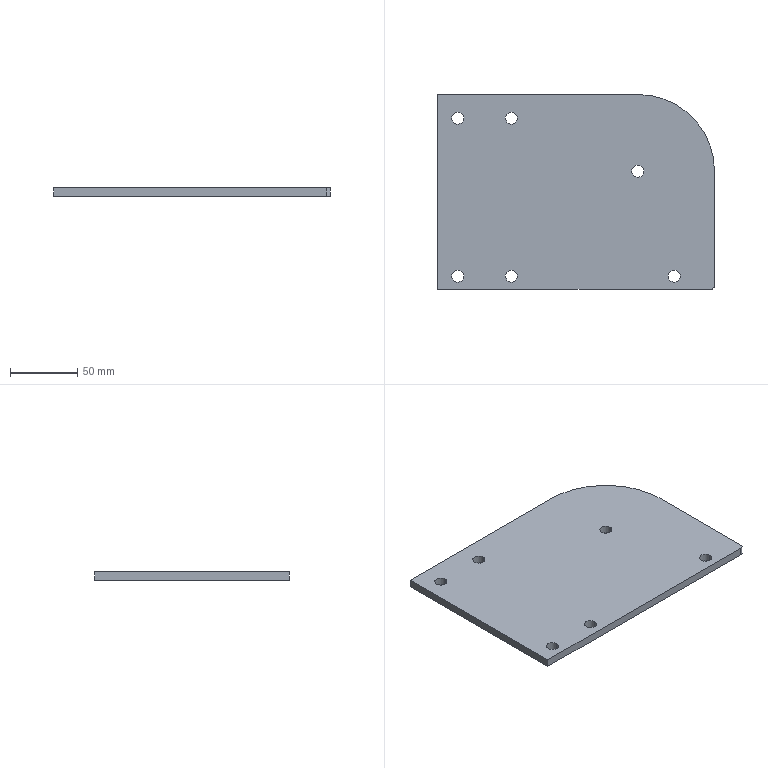Part | SolidWorks | features ICE 7, Fillet 6, Chamfer 1, Extrusion 1, HoleWzd 1 | 1 solid | 20 faces | box 206 x 145 x 6 mm | volume 172735 mm3 | cylinder 14 | plane 6 | commonest cylinder face diameters 9 x12 6 x1 114 x1
STEP:
#1=CARTESIAN_POINT('',(68.5,-62.5,6.));
#2=VERTEX_POINT('',#1);
#3=CARTESIAN_POINT('',(77.5,-62.5,6.));
#4=VERTEX_POINT('',#3);
#5=CARTESIAN_POINT('',(73.,-62.5,6.));
#6=DIRECTION('',(0.,0.,1.));
#7=DIRECTION('',(1.,0.,0.));
#8=AXIS2_PLACEMENT_3D('',#5,#6,#7);
#9=CIRCLE('',#8,4.5);
#10=EDGE_CURVE('',#2,#4,#9,.T.);
#11=ORIENTED_EDGE('',*,*,#10,.T.);
#12=CARTESIAN_POINT('',(77.5,-62.5,0.));
#13=VERTEX_POINT('',#12);
#14=CARTESIAN_POINT('',(77.5,-62.5,10.));
#15=DIRECTION('',(0.,0.,-1.));
#16=VECTOR('',#15,1000.);
#17=LINE('',#14,#16);
#18=EDGE_CURVE('',#4,#13,#17,.T.);
#19=ORIENTED_EDGE('',*,*,#18,.T.);
#20=CARTESIAN_POINT('',(68.5,-62.5,0.));
#21=VERTEX_POINT('',#20);
#22=CARTESIAN_POINT('',(73.,-62.5,0.));
#23=DIRECTION('',(0.,0.,-1.));
#24=DIRECTION('',(-1.,0.,0.));
#25=AXIS2_PLACEMENT_3D('',#22,#23,#24);
#26=CIRCLE('',#25,4.5);
#27=EDGE_CURVE('',#13,#21,#26,.T.);
#28=ORIENTED_EDGE('',*,*,#27,.T.);
#29=CARTESIAN_POINT('',(68.5,-62.5,10.));
#30=DIRECTION('',(0.,0.,-1.));
#31=VECTOR('',#30,1000.);
#32=LINE('',#29,#31);
#33=EDGE_CURVE('',#2,#21,#32,.T.);
#34=ORIENTED_EDGE('',*,*,#33,.F.);
#35=EDGE_LOOP('',(#11,#19,#28,#34));
#36=FACE_OUTER_BOUND('',#35,.T.);
#37=CARTESIAN_POINT('',(73.,-62.5,10.));
#38=DIRECTION('',(0.,0.,-1.));
#39=DIRECTION('',(-1.,0.,0.));
#40=AXIS2_PLACEMENT_3D('',#37,#38,#39);
#41=CYLINDRICAL_SURFACE('',#40,4.5);
#42=ADVANCED_FACE('',(#36),#41,.F.);
#43=CARTESIAN_POINT('',(41.5,15.5,0.));
#44=VERTEX_POINT('',#43);
#45=CARTESIAN_POINT('',(50.5,15.5,0.));
#46=VERTEX_POINT('',#45);
#47=CARTESIAN_POINT('',(46.,15.5,0.));
#48=DIRECTION('',(0.,0.,1.));
#49=DIRECTION('',(1.,0.,0.));
#50=AXIS2_PLACEMENT_3D('',#47,#48,#49);
#51=CIRCLE('',#50,4.5);
#52=EDGE_CURVE('',#44,#46,#51,.T.);
#53=ORIENTED_EDGE('',*,*,#52,.F.);
#54=CARTESIAN_POINT('',(41.5,15.5,6.));
#55=VERTEX_POINT('',#54);
#56=CARTESIAN_POINT('',(41.5,15.5,0.));
#57=DIRECTION('',(0.,0.,1.));
#58=VECTOR('',#57,1000.);
#59=LINE('',#56,#58);
#60=EDGE_CURVE('',#44,#55,#59,.T.);
#61=ORIENTED_EDGE('',*,*,#60,.T.);
#62=CARTESIAN_POINT('',(50.5,15.5,6.));
#63=VERTEX_POINT('',#62);
#64=CARTESIAN_POINT('',(46.,15.5,6.));
#65=DIRECTION('',(0.,0.,1.));
#66=DIRECTION('',(1.,0.,0.));
#67=AXIS2_PLACEMENT_3D('',#64,#65,#66);
#68=CIRCLE('',#67,4.5);
#69=EDGE_CURVE('',#55,#63,#68,.T.);
#70=ORIENTED_EDGE('',*,*,#69,.T.);
#71=CARTESIAN_POINT('',(50.5,15.5,0.));
#72=DIRECTION('',(0.,0.,1.));
#73=VECTOR('',#72,1000.);
#74=LINE('',#71,#73);
#75=EDGE_CURVE('',#46,#63,#74,.T.);
#76=ORIENTED_EDGE('',*,*,#75,.F.);
#77=EDGE_LOOP('',(#53,#61,#70,#76));
#78=FACE_OUTER_BOUND('',#77,.T.);
#79=CARTESIAN_POINT('',(46.,15.5,0.));
#80=DIRECTION('',(0.,0.,1.));
#81=DIRECTION('',(1.,0.,0.));
#82=AXIS2_PLACEMENT_3D('',#79,#80,#81);
#83=CYLINDRICAL_SURFACE('',#82,4.5);
#84=ADVANCED_FACE('',(#78),#83,.F.);
#85=CARTESIAN_POINT('',(-52.5,-62.5,0.));
#86=VERTEX_POINT('',#85);
#87=CARTESIAN_POINT('',(-43.5,-62.5,0.));
#88=VERTEX_POINT('',#87);
#89=CARTESIAN_POINT('',(-48.,-62.5,0.));
#90=DIRECTION('',(0.,0.,1.));
#91=DIRECTION('',(1.,0.,0.));
#92=AXIS2_PLACEMENT_3D('',#89,#90,#91);
#93=CIRCLE('',#92,4.5);
#94=EDGE_CURVE('',#86,#88,#93,.T.);
#95=ORIENTED_EDGE('',*,*,#94,.F.);
#96=CARTESIAN_POINT('',(-52.5,-62.5,6.));
#97=VERTEX_POINT('',#96);
#98=CARTESIAN_POINT('',(-52.5,-62.5,0.));
#99=DIRECTION('',(0.,0.,1.));
#100=VECTOR('',#99,1000.);
#101=LINE('',#98,#100);
#102=EDGE_CURVE('',#86,#97,#101,.T.);
#103=ORIENTED_EDGE('',*,*,#102,.T.);
#104=CARTESIAN_POINT('',(-43.5,-62.5,6.));
#105=VERTEX_POINT('',#104);
#106=CARTESIAN_POINT('',(-48.,-62.5,6.));
#107=DIRECTION('',(0.,0.,1.));
#108=DIRECTION('',(1.,0.,0.));
#109=AXIS2_PLACEMENT_3D('',#106,#107,#108);
#110=CIRCLE('',#109,4.5);
#111=EDGE_CURVE('',#97,#105,#110,.T.);
#112=ORIENTED_EDGE('',*,*,#111,.T.);
#113=CARTESIAN_POINT('',(-43.5,-62.5,0.));
#114=DIRECTION('',(0.,0.,1.));
#115=VECTOR('',#114,1000.);
#116=LINE('',#113,#115);
#117=EDGE_CURVE('',#88,#105,#116,.T.);
#118=ORIENTED_EDGE('',*,*,#117,.F.);
#119=EDGE_LOOP('',(#95,#103,#112,#118));
#120=FACE_OUTER_BOUND('',#119,.T.);
#121=CARTESIAN_POINT('',(-48.,-62.5,0.));
#122=DIRECTION('',(0.,0.,1.));
#123=DIRECTION('',(1.,0.,0.));
#124=AXIS2_PLACEMENT_3D('',#121,#122,#123);
#125=CYLINDRICAL_SURFACE('',#124,4.5);
#126=ADVANCED_FACE('',(#120),#125,.F.);
#127=CARTESIAN_POINT('',(-92.5,-62.5,0.));
#128=VERTEX_POINT('',#127);
#129=CARTESIAN_POINT('',(-83.5,-62.5,0.));
#130=VERTEX_POINT('',#129);
#131=CARTESIAN_POINT('',(-88.,-62.5,0.));
#132=DIRECTION('',(0.,0.,1.));
#133=DIRECTION('',(1.,0.,0.));
#134=AXIS2_PLACEMENT_3D('',#131,#132,#133);
#135=CIRCLE('',#134,4.5);
#136=EDGE_CURVE('',#128,#130,#135,.T.);
#137=ORIENTED_EDGE('',*,*,#136,.F.);
#138=CARTESIAN_POINT('',(-92.5,-62.5,6.));
#139=VERTEX_POINT('',#138);
#140=CARTESIAN_POINT('',(-92.5,-62.5,0.));
#141=DIRECTION('',(0.,0.,1.));
#142=VECTOR('',#141,1000.);
#143=LINE('',#140,#142);
#144=EDGE_CURVE('',#128,#139,#143,.T.);
#145=ORIENTED_EDGE('',*,*,#144,.T.);
#146=CARTESIAN_POINT('',(-83.5,-62.5,6.));
#147=VERTEX_POINT('',#146);
#148=CARTESIAN_POINT('',(-88.,-62.5,6.));
#149=DIRECTION('',(0.,0.,1.));
#150=DIRECTION('',(1.,0.,0.));
#151=AXIS2_PLACEMENT_3D('',#148,#149,#150);
#152=CIRCLE('',#151,4.5);
#153=EDGE_CURVE('',#139,#147,#152,.T.);
#154=ORIENTED_EDGE('',*,*,#153,.T.);
#155=CARTESIAN_POINT('',(-83.5,-62.5,0.));
#156=DIRECTION('',(0.,0.,1.));
#157=VECTOR('',#156,1000.);
#158=LINE('',#155,#157);
#159=EDGE_CURVE('',#130,#147,#158,.T.);
#160=ORIENTED_EDGE('',*,*,#159,.F.);
#161=EDGE_LOOP('',(#137,#145,#154,#160));
#162=FACE_OUTER_BOUND('',#161,.T.);
#163=CARTESIAN_POINT('',(-88.,-62.5,0.));
#164=DIRECTION('',(0.,0.,1.));
#165=DIRECTION('',(1.,0.,0.));
#166=AXIS2_PLACEMENT_3D('',#163,#164,#165);
#167=CYLINDRICAL_SURFACE('',#166,4.5);
#168=ADVANCED_FACE('',(#162),#167,.F.);
#169=CARTESIAN_POINT('',(-52.5,55.,0.));
#170=VERTEX_POINT('',#169);
#171=CARTESIAN_POINT('',(-43.5,55.,0.));
#172=VERTEX_POINT('',#171);
#173=CARTESIAN_POINT('',(-48.,55.,0.));
#174=DIRECTION('',(0.,0.,1.));
#175=DIRECTION('',(1.,0.,0.));
#176=AXIS2_PLACEMENT_3D('',#173,#174,#175);
#177=CIRCLE('',#176,4.5);
#178=EDGE_CURVE('',#170,#172,#177,.T.);
#179=ORIENTED_EDGE('',*,*,#178,.F.);
#180=CARTESIAN_POINT('',(-52.5,55.,6.));
#181=VERTEX_POINT('',#180);
#182=CARTESIAN_POINT('',(-52.5,55.,0.));
#183=DIRECTION('',(0.,0.,1.));
#184=VECTOR('',#183,1000.);
#185=LINE('',#182,#184);
#186=EDGE_CURVE('',#170,#181,#185,.T.);
#187=ORIENTED_EDGE('',*,*,#186,.T.);
#188=CARTESIAN_POINT('',(-43.5,55.,6.));
#189=VERTEX_POINT('',#188);
#190=CARTESIAN_POINT('',(-48.,55.,6.));
#191=DIRECTION('',(0.,0.,1.));
#192=DIRECTION('',(1.,0.,0.));
#193=AXIS2_PLACEMENT_3D('',#190,#191,#192);
#194=CIRCLE('',#193,4.5);
#195=EDGE_CURVE('',#181,#189,#194,.T.);
#196=ORIENTED_EDGE('',*,*,#195,.T.);
#197=CARTESIAN_POINT('',(-43.5,55.,0.));
#198=DIRECTION('',(0.,0.,1.));
#199=VECTOR('',#198,1000.);
#200=LINE('',#197,#199);
#201=EDGE_CURVE('',#172,#189,#200,.T.);
#202=ORIENTED_EDGE('',*,*,#201,.F.);
#203=EDGE_LOOP('',(#179,#187,#196,#202));
#204=FACE_OUTER_BOUND('',#203,.T.);
#205=CARTESIAN_POINT('',(-48.,55.,0.));
#206=DIRECTION('',(0.,0.,1.));
#207=DIRECTION('',(1.,0.,0.));
#208=AXIS2_PLACEMENT_3D('',#205,#206,#207);
#209=CYLINDRICAL_SURFACE('',#208,4.5);
#210=ADVANCED_FACE('',(#204),#209,.F.);
#211=CARTESIAN_POINT('',(-92.5,55.,0.));
#212=VERTEX_POINT('',#211);
#213=CARTESIAN_POINT('',(-83.5,55.,0.));
#214=VERTEX_POINT('',#213);
#215=CARTESIAN_POINT('',(-88.,55.,0.));
#216=DIRECTION('',(0.,0.,1.));
#217=DIRECTION('',(1.,0.,0.));
#218=AXIS2_PLACEMENT_3D('',#215,#216,#217);
#219=CIRCLE('',#218,4.5);
#220=EDGE_CURVE('',#212,#214,#219,.T.);
#221=ORIENTED_EDGE('',*,*,#220,.F.);
#222=CARTESIAN_POINT('',(-92.5,55.,6.));
#223=VERTEX_POINT('',#222);
#224=CARTESIAN_POINT('',(-92.5,55.,0.));
#225=DIRECTION('',(0.,0.,1.));
#226=VECTOR('',#225,1000.);
#227=LINE('',#224,#226);
#228=EDGE_CURVE('',#212,#223,#227,.T.);
#229=ORIENTED_EDGE('',*,*,#228,.T.);
#230=CARTESIAN_POINT('',(-83.5,55.,6.));
#231=VERTEX_POINT('',#230);
#232=CARTESIAN_POINT('',(-88.,55.,6.));
#233=DIRECTION('',(0.,0.,1.));
#234=DIRECTION('',(1.,0.,0.));
#235=AXIS2_PLACEMENT_3D('',#232,#233,#234);
#236=CIRCLE('',#235,4.5);
#237=EDGE_CURVE('',#223,#231,#236,.T.);
#238=ORIENTED_EDGE('',*,*,#237,.T.);
#239=CARTESIAN_POINT('',(-83.5,55.,0.));
#240=DIRECTION('',(0.,0.,1.));
#241=VECTOR('',#240,1000.);
#242=LINE('',#239,#241);
#243=EDGE_CURVE('',#214,#231,#242,.T.);
#244=ORIENTED_EDGE('',*,*,#243,.F.);
#245=EDGE_LOOP('',(#221,#229,#238,#244));
#246=FACE_OUTER_BOUND('',#245,.T.);
#247=CARTESIAN_POINT('',(-88.,55.,0.));
#248=DIRECTION('',(0.,0.,1.));
#249=DIRECTION('',(1.,0.,0.));
#250=AXIS2_PLACEMENT_3D('',#247,#248,#249);
#251=CYLINDRICAL_SURFACE('',#250,4.5);
#252=ADVANCED_FACE('',(#246),#251,.F.);
#253=CARTESIAN_POINT('',(-103.,72.5,0.));
#254=VERTEX_POINT('',#253);
#255=CARTESIAN_POINT('',(-103.,-72.5,0.));
#256=VERTEX_POINT('',#255);
#257=CARTESIAN_POINT('',(-103.,72.5,0.));
#258=DIRECTION('',(0.,-1.,0.));
#259=VECTOR('',#258,1000.);
#260=LINE('',#257,#259);
#261=EDGE_CURVE('',#254,#256,#260,.T.);
#262=ORIENTED_EDGE('',*,*,#261,.T.);
#263=CARTESIAN_POINT('',(-103.,-72.5,6.));
#264=VERTEX_POINT('',#263);
#265=CARTESIAN_POINT('',(-103.,-72.5,6.));
#266=DIRECTION('',(0.,0.,-1.));
#267=VECTOR('',#266,1000.);
#268=LINE('',#265,#267);
#269=EDGE_CURVE('',#264,#256,#268,.T.);
#270=ORIENTED_EDGE('',*,*,#269,.F.);
#271=CARTESIAN_POINT('',(-103.,72.5,6.));
#272=VERTEX_POINT('',#271);
#273=CARTESIAN_POINT('',(-103.,72.5,6.));
#274=DIRECTION('',(0.,-1.,0.));
#275=VECTOR('',#274,1000.);
#276=LINE('',#273,#275);
#277=EDGE_CURVE('',#272,#264,#276,.T.);
#278=ORIENTED_EDGE('',*,*,#277,.F.);
#279=CARTESIAN_POINT('',(-103.,72.5,6.));
#280=DIRECTION('',(0.,0.,-1.));
#281=VECTOR('',#280,1000.);
#282=LINE('',#279,#281);
#283=EDGE_CURVE('',#272,#254,#282,.T.);
#284=ORIENTED_EDGE('',*,*,#283,.T.);
#285=EDGE_LOOP('',(#262,#270,#278,#284));
#286=FACE_OUTER_BOUND('',#285,.T.);
#287=CARTESIAN_POINT('',(-103.,72.5,6.));
#288=DIRECTION('',(1.,0.,0.));
#289=DIRECTION('',(0.,0.,-1.));
#290=AXIS2_PLACEMENT_3D('',#287,#288,#289);
#291=PLANE('',#290);
#292=ADVANCED_FACE('',(#286),#291,.F.);
#293=CARTESIAN_POINT('',(100.,-72.5,0.));
#294=VERTEX_POINT('',#293);
#295=CARTESIAN_POINT('',(-103.,-72.5,0.));
#296=DIRECTION('',(1.,0.,0.));
#297=VECTOR('',#296,1000.);
#298=LINE('',#295,#297);
#299=EDGE_CURVE('',#256,#294,#298,.T.);
#300=ORIENTED_EDGE('',*,*,#299,.T.);
#301=CARTESIAN_POINT('',(100.,-72.5,6.));
#302=VERTEX_POINT('',#301);
#303=CARTESIAN_POINT('',(100.,-72.5,6.));
#304=DIRECTION('',(0.,0.,1.));
#305=VECTOR('',#304,1000.);
#306=LINE('',#303,#305);
#307=EDGE_CURVE('',#294,#302,#306,.T.);
#308=ORIENTED_EDGE('',*,*,#307,.T.);
#309=CARTESIAN_POINT('',(-103.,-72.5,6.));
#310=DIRECTION('',(1.,0.,0.));
#311=VECTOR('',#310,1000.);
#312=LINE('',#309,#311);
#313=EDGE_CURVE('',#264,#302,#312,.T.);
#314=ORIENTED_EDGE('',*,*,#313,.F.);
#315=ORIENTED_EDGE('',*,*,#269,.T.);
#316=EDGE_LOOP('',(#300,#308,#314,#315));
#317=FACE_OUTER_BOUND('',#316,.T.);
#318=CARTESIAN_POINT('',(-103.,-72.5,6.));
#319=DIRECTION('',(0.,1.,0.));
#320=DIRECTION('',(0.,0.,1.));
#321=AXIS2_PLACEMENT_3D('',#318,#319,#320);
#322=PLANE('',#321);
#323=ADVANCED_FACE('',(#317),#322,.F.);
#324=CARTESIAN_POINT('',(103.,-69.5,6.));
#325=VERTEX_POINT('',#324);
#326=CARTESIAN_POINT('',(103.,15.5,6.));
#327=VERTEX_POINT('',#326);
#328=CARTESIAN_POINT('',(103.,72.5,6.));
#329=DIRECTION('',(0.,1.,0.));
#330=VECTOR('',#329,1000.);
#331=LINE('',#328,#330);
#332=EDGE_CURVE('',#325,#327,#331,.T.);
#333=ORIENTED_EDGE('',*,*,#332,.F.);
#334=CARTESIAN_POINT('',(103.,-69.5,0.));
#335=VERTEX_POINT('',#334);
#336=CARTESIAN_POINT('',(103.,-69.5,6.));
#337=DIRECTION('',(0.,0.,-1.));
#338=VECTOR('',#337,1000.);
#339=LINE('',#336,#338);
#340=EDGE_CURVE('',#325,#335,#339,.T.);
#341=ORIENTED_EDGE('',*,*,#340,.T.);
#342=CARTESIAN_POINT('',(103.,15.5,0.));
#343=VERTEX_POINT('',#342);
#344=CARTESIAN_POINT('',(103.,72.5,0.));
#345=DIRECTION('',(0.,1.,0.));
#346=VECTOR('',#345,1000.);
#347=LINE('',#344,#346);
#348=EDGE_CURVE('',#335,#343,#347,.T.);
#349=ORIENTED_EDGE('',*,*,#348,.T.);
#350=CARTESIAN_POINT('',(103.,15.5,6.));
#351=DIRECTION('',(0.,0.,1.));
#352=VECTOR('',#351,1000.);
#353=LINE('',#350,#352);
#354=EDGE_CURVE('',#343,#327,#353,.T.);
#355=ORIENTED_EDGE('',*,*,#354,.T.);
#356=EDGE_LOOP('',(#333,#341,#349,#355));
#357=FACE_OUTER_BOUND('',#356,.T.);
#358=CARTESIAN_POINT('',(103.,72.5,6.));
#359=DIRECTION('',(-1.,0.,0.));
#360=DIRECTION('',(0.,0.,1.));
#361=AXIS2_PLACEMENT_3D('',#358,#359,#360);
#362=PLANE('',#361);
#363=ADVANCED_FACE('',(#357),#362,.F.);
#364=CARTESIAN_POINT('',(46.,72.5,6.));
#365=VERTEX_POINT('',#364);
#366=CARTESIAN_POINT('',(-103.,72.5,6.));
#367=DIRECTION('',(-1.,0.,0.));
#368=VECTOR('',#367,1000.);
#369=LINE('',#366,#368);
#370=EDGE_CURVE('',#365,#272,#369,.T.);
#371=ORIENTED_EDGE('',*,*,#370,.F.);
#372=CARTESIAN_POINT('',(46.,72.5,0.));
#373=VERTEX_POINT('',#372);
#374=CARTESIAN_POINT('',(46.,72.5,6.));
#375=DIRECTION('',(0.,0.,-1.));
#376=VECTOR('',#375,1000.);
#377=LINE('',#374,#376);
#378=EDGE_CURVE('',#365,#373,#377,.T.);
#379=ORIENTED_EDGE('',*,*,#378,.T.);
#380=CARTESIAN_POINT('',(-103.,72.5,0.));
#381=DIRECTION('',(-1.,0.,0.));
#382=VECTOR('',#381,1000.);
#383=LINE('',#380,#382);
#384=EDGE_CURVE('',#373,#254,#383,.T.);
#385=ORIENTED_EDGE('',*,*,#384,.T.);
#386=ORIENTED_EDGE('',*,*,#283,.F.);
#387=EDGE_LOOP('',(#371,#379,#385,#386));
#388=FACE_OUTER_BOUND('',#387,.T.);
#389=CARTESIAN_POINT('',(-103.,72.5,6.));
#390=DIRECTION('',(0.,-1.,0.));
#391=DIRECTION('',(0.,0.,-1.));
#392=AXIS2_PLACEMENT_3D('',#389,#390,#391);
#393=PLANE('',#392);
#394=ADVANCED_FACE('',(#388),#393,.F.);
#395=ORIENTED_EDGE('',*,*,#10,.F.);
#396=CARTESIAN_POINT('',(73.,-62.5,6.));
#397=DIRECTION('',(0.,0.,1.));
#398=DIRECTION('',(1.,0.,0.));
#399=AXIS2_PLACEMENT_3D('',#396,#397,#398);
#400=CIRCLE('',#399,4.5);
#401=EDGE_CURVE('',#4,#2,#400,.T.);
#402=ORIENTED_EDGE('',*,*,#401,.F.);
#403=EDGE_LOOP('',(#395,#402));
#404=FACE_BOUND('',#403,.T.);
#405=CARTESIAN_POINT('',(46.,15.5,6.));
#406=DIRECTION('',(0.,0.,1.));
#407=DIRECTION('',(1.,0.,0.));
#408=AXIS2_PLACEMENT_3D('',#405,#406,#407);
#409=CIRCLE('',#408,4.5);
#410=EDGE_CURVE('',#63,#55,#409,.T.);
#411=ORIENTED_EDGE('',*,*,#410,.F.);
#412=ORIENTED_EDGE('',*,*,#69,.F.);
#413=EDGE_LOOP('',(#411,#412));
#414=FACE_BOUND('',#413,.T.);
#415=CARTESIAN_POINT('',(-48.,-62.5,6.));
#416=DIRECTION('',(0.,0.,1.));
#417=DIRECTION('',(1.,0.,0.));
#418=AXIS2_PLACEMENT_3D('',#415,#416,#417);
#419=CIRCLE('',#418,4.5);
#420=EDGE_CURVE('',#105,#97,#419,.T.);
#421=ORIENTED_EDGE('',*,*,#420,.F.);
#422=ORIENTED_EDGE('',*,*,#111,.F.);
#423=EDGE_LOOP('',(#421,#422));
#424=FACE_BOUND('',#423,.T.);
#425=CARTESIAN_POINT('',(-88.,-62.5,6.));
#426=DIRECTION('',(0.,0.,1.));
#427=DIRECTION('',(1.,0.,0.));
#428=AXIS2_PLACEMENT_3D('',#425,#426,#427);
#429=CIRCLE('',#428,4.5);
#430=EDGE_CURVE('',#147,#139,#429,.T.);
#431=ORIENTED_EDGE('',*,*,#430,.F.);
#432=ORIENTED_EDGE('',*,*,#153,.F.);
#433=EDGE_LOOP('',(#431,#432));
#434=FACE_BOUND('',#433,.T.);
#435=CARTESIAN_POINT('',(-48.,55.,6.));
#436=DIRECTION('',(0.,0.,1.));
#437=DIRECTION('',(1.,0.,0.));
#438=AXIS2_PLACEMENT_3D('',#435,#436,#437);
#439=CIRCLE('',#438,4.5);
#440=EDGE_CURVE('',#189,#181,#439,.T.);
#441=ORIENTED_EDGE('',*,*,#440,.F.);
#442=ORIENTED_EDGE('',*,*,#195,.F.);
#443=EDGE_LOOP('',(#441,#442));
#444=FACE_BOUND('',#443,.T.);
#445=CARTESIAN_POINT('',(-88.,55.,6.));
#446=DIRECTION('',(0.,0.,1.));
#447=DIRECTION('',(1.,0.,0.));
#448=AXIS2_PLACEMENT_3D('',#445,#446,#447);
#449=CIRCLE('',#448,4.5);
#450=EDGE_CURVE('',#231,#223,#449,.T.);
#451=ORIENTED_EDGE('',*,*,#450,.F.);
#452=ORIENTED_EDGE('',*,*,#237,.F.);
#453=EDGE_LOOP('',(#451,#452));
#454=FACE_BOUND('',#453,.T.);
#455=ORIENTED_EDGE('',*,*,#313,.T.);
#456=CARTESIAN_POINT('',(100.,-69.5,6.));
#457=DIRECTION('',(0.,0.,1.));
#458=DIRECTION('',(1.,0.,0.));
#459=AXIS2_PLACEMENT_3D('',#456,#457,#458);
#460=CIRCLE('',#459,3.);
#461=EDGE_CURVE('',#302,#325,#460,.T.);
#462=ORIENTED_EDGE('',*,*,#461,.T.);
#463=ORIENTED_EDGE('',*,*,#332,.T.);
#464=CARTESIAN_POINT('',(46.,15.5,6.));
#465=DIRECTION('',(0.,0.,1.));
#466=DIRECTION('',(1.,0.,0.));
#467=AXIS2_PLACEMENT_3D('',#464,#465,#466);
#468=CIRCLE('',#467,57.);
#469=EDGE_CURVE('',#327,#365,#468,.T.);
#470=ORIENTED_EDGE('',*,*,#469,.T.);
#471=ORIENTED_EDGE('',*,*,#370,.T.);
#472=ORIENTED_EDGE('',*,*,#277,.T.);
#473=EDGE_LOOP('',(#455,#462,#463,#470,#471,#472));
#474=FACE_OUTER_BOUND('',#473,.T.);
#475=CARTESIAN_POINT('',(0.,0.,6.));
#476=DIRECTION('',(0.,0.,1.));
#477=DIRECTION('',(1.,0.,0.));
#478=AXIS2_PLACEMENT_3D('',#475,#476,#477);
#479=PLANE('',#478);
#480=ADVANCED_FACE('',(#404,#414,#424,#434,#444,#454,#474),#479,.T.);
#481=CARTESIAN_POINT('',(73.,-62.5,0.));
#482=DIRECTION('',(0.,0.,-1.));
#483=DIRECTION('',(-1.,0.,0.));
#484=AXIS2_PLACEMENT_3D('',#481,#482,#483);
#485=CIRCLE('',#484,4.5);
#486=EDGE_CURVE('',#21,#13,#485,.T.);
#487=ORIENTED_EDGE('',*,*,#486,.F.);
#488=ORIENTED_EDGE('',*,*,#27,.F.);
#489=EDGE_LOOP('',(#487,#488));
#490=FACE_BOUND('',#489,.T.);
#491=CARTESIAN_POINT('',(46.,15.5,0.));
#492=DIRECTION('',(0.,0.,1.));
#493=DIRECTION('',(1.,0.,0.));
#494=AXIS2_PLACEMENT_3D('',#491,#492,#493);
#495=CIRCLE('',#494,4.5);
#496=EDGE_CURVE('',#46,#44,#495,.T.);
#497=ORIENTED_EDGE('',*,*,#496,.T.);
#498=ORIENTED_EDGE('',*,*,#52,.T.);
#499=EDGE_LOOP('',(#497,#498));
#500=FACE_BOUND('',#499,.T.);
#501=CARTESIAN_POINT('',(-48.,-62.5,0.));
#502=DIRECTION('',(0.,0.,1.));
#503=DIRECTION('',(1.,0.,0.));
#504=AXIS2_PLACEMENT_3D('',#501,#502,#503);
#505=CIRCLE('',#504,4.5);
#506=EDGE_CURVE('',#88,#86,#505,.T.);
#507=ORIENTED_EDGE('',*,*,#506,.T.);
#508=ORIENTED_EDGE('',*,*,#94,.T.);
#509=EDGE_LOOP('',(#507,#508));
#510=FACE_BOUND('',#509,.T.);
#511=CARTESIAN_POINT('',(-88.,-62.5,0.));
#512=DIRECTION('',(0.,0.,1.));
#513=DIRECTION('',(1.,0.,0.));
#514=AXIS2_PLACEMENT_3D('',#511,#512,#513);
#515=CIRCLE('',#514,4.5);
#516=EDGE_CURVE('',#130,#128,#515,.T.);
#517=ORIENTED_EDGE('',*,*,#516,.T.);
#518=ORIENTED_EDGE('',*,*,#136,.T.);
#519=EDGE_LOOP('',(#517,#518));
#520=FACE_BOUND('',#519,.T.);
#521=CARTESIAN_POINT('',(-48.,55.,0.));
#522=DIRECTION('',(0.,0.,1.));
#523=DIRECTION('',(1.,0.,0.));
#524=AXIS2_PLACEMENT_3D('',#521,#522,#523);
#525=CIRCLE('',#524,4.5);
#526=EDGE_CURVE('',#172,#170,#525,.T.);
#527=ORIENTED_EDGE('',*,*,#526,.T.);
#528=ORIENTED_EDGE('',*,*,#178,.T.);
#529=EDGE_LOOP('',(#527,#528));
#530=FACE_BOUND('',#529,.T.);
#531=CARTESIAN_POINT('',(-88.,55.,0.));
#532=DIRECTION('',(0.,0.,1.));
#533=DIRECTION('',(1.,0.,0.));
#534=AXIS2_PLACEMENT_3D('',#531,#532,#533);
#535=CIRCLE('',#534,4.5);
#536=EDGE_CURVE('',#214,#212,#535,.T.);
#537=ORIENTED_EDGE('',*,*,#536,.T.);
#538=ORIENTED_EDGE('',*,*,#220,.T.);
#539=EDGE_LOOP('',(#537,#538));
#540=FACE_BOUND('',#539,.T.);
#541=ORIENTED_EDGE('',*,*,#348,.F.);
#542=CARTESIAN_POINT('',(100.,-69.5,0.));
#543=DIRECTION('',(0.,0.,-1.));
#544=DIRECTION('',(1.,0.,0.));
#545=AXIS2_PLACEMENT_3D('',#542,#543,#544);
#546=CIRCLE('',#545,3.);
#547=EDGE_CURVE('',#335,#294,#546,.T.);
#548=ORIENTED_EDGE('',*,*,#547,.T.);
#549=ORIENTED_EDGE('',*,*,#299,.F.);
#550=ORIENTED_EDGE('',*,*,#261,.F.);
#551=ORIENTED_EDGE('',*,*,#384,.F.);
#552=CARTESIAN_POINT('',(46.,15.5,0.));
#553=DIRECTION('',(0.,0.,-1.));
#554=DIRECTION('',(1.,0.,0.));
#555=AXIS2_PLACEMENT_3D('',#552,#553,#554);
#556=CIRCLE('',#555,57.);
#557=EDGE_CURVE('',#373,#343,#556,.T.);
#558=ORIENTED_EDGE('',*,*,#557,.T.);
#559=EDGE_LOOP('',(#541,#548,#549,#550,#551,#558));
#560=FACE_OUTER_BOUND('',#559,.T.);
#561=CARTESIAN_POINT('',(0.,0.,0.));
#562=DIRECTION('',(0.,0.,1.));
#563=DIRECTION('',(1.,0.,0.));
#564=AXIS2_PLACEMENT_3D('',#561,#562,#563);
#565=PLANE('',#564);
#566=ADVANCED_FACE('',(#490,#500,#510,#520,#530,#540,#560),#565,.F.);
#567=ORIENTED_EDGE('',*,*,#228,.F.);
#568=ORIENTED_EDGE('',*,*,#536,.F.);
#569=ORIENTED_EDGE('',*,*,#243,.T.);
#570=ORIENTED_EDGE('',*,*,#450,.T.);
#571=EDGE_LOOP('',(#567,#568,#569,#570));
#572=FACE_OUTER_BOUND('',#571,.T.);
#573=CARTESIAN_POINT('',(-88.,55.,0.));
#574=DIRECTION('',(0.,0.,1.));
#575=DIRECTION('',(1.,0.,0.));
#576=AXIS2_PLACEMENT_3D('',#573,#574,#575);
#577=CYLINDRICAL_SURFACE('',#576,4.5);
#578=ADVANCED_FACE('',(#572),#577,.F.);
#579=ORIENTED_EDGE('',*,*,#186,.F.);
#580=ORIENTED_EDGE('',*,*,#526,.F.);
#581=ORIENTED_EDGE('',*,*,#201,.T.);
#582=ORIENTED_EDGE('',*,*,#440,.T.);
#583=EDGE_LOOP('',(#579,#580,#581,#582));
#584=FACE_OUTER_BOUND('',#583,.T.);
#585=CARTESIAN_POINT('',(-48.,55.,0.));
#586=DIRECTION('',(0.,0.,1.));
#587=DIRECTION('',(1.,0.,0.));
#588=AXIS2_PLACEMENT_3D('',#585,#586,#587);
#589=CYLINDRICAL_SURFACE('',#588,4.5);
#590=ADVANCED_FACE('',(#584),#589,.F.);
#591=ORIENTED_EDGE('',*,*,#144,.F.);
#592=ORIENTED_EDGE('',*,*,#516,.F.);
#593=ORIENTED_EDGE('',*,*,#159,.T.);
#594=ORIENTED_EDGE('',*,*,#430,.T.);
#595=EDGE_LOOP('',(#591,#592,#593,#594));
#596=FACE_OUTER_BOUND('',#595,.T.);
#597=CARTESIAN_POINT('',(-88.,-62.5,0.));
#598=DIRECTION('',(0.,0.,1.));
#599=DIRECTION('',(1.,0.,0.));
#600=AXIS2_PLACEMENT_3D('',#597,#598,#599);
#601=CYLINDRICAL_SURFACE('',#600,4.5);
#602=ADVANCED_FACE('',(#596),#601,.F.);
#603=ORIENTED_EDGE('',*,*,#102,.F.);
#604=ORIENTED_EDGE('',*,*,#506,.F.);
#605=ORIENTED_EDGE('',*,*,#117,.T.);
#606=ORIENTED_EDGE('',*,*,#420,.T.);
#607=EDGE_LOOP('',(#603,#604,#605,#606));
#608=FACE_OUTER_BOUND('',#607,.T.);
#609=CARTESIAN_POINT('',(-48.,-62.5,0.));
#610=DIRECTION('',(0.,0.,1.));
#611=DIRECTION('',(1.,0.,0.));
#612=AXIS2_PLACEMENT_3D('',#609,#610,#611);
#613=CYLINDRICAL_SURFACE('',#612,4.5);
#614=ADVANCED_FACE('',(#608),#613,.F.);
#615=ORIENTED_EDGE('',*,*,#60,.F.);
#616=ORIENTED_EDGE('',*,*,#496,.F.);
#617=ORIENTED_EDGE('',*,*,#75,.T.);
#618=ORIENTED_EDGE('',*,*,#410,.T.);
#619=EDGE_LOOP('',(#615,#616,#617,#618));
#620=FACE_OUTER_BOUND('',#619,.T.);
#621=CARTESIAN_POINT('',(46.,15.5,0.));
#622=DIRECTION('',(0.,0.,1.));
#623=DIRECTION('',(1.,0.,0.));
#624=AXIS2_PLACEMENT_3D('',#621,#622,#623);
#625=CYLINDRICAL_SURFACE('',#624,4.5);
#626=ADVANCED_FACE('',(#620),#625,.F.);
#627=ORIENTED_EDGE('',*,*,#469,.F.);
#628=ORIENTED_EDGE('',*,*,#354,.F.);
#629=ORIENTED_EDGE('',*,*,#557,.F.);
#630=ORIENTED_EDGE('',*,*,#378,.F.);
#631=EDGE_LOOP('',(#627,#628,#629,#630));
#632=FACE_OUTER_BOUND('',#631,.T.);
#633=CARTESIAN_POINT('',(46.,15.5,6.));
#634=DIRECTION('',(0.,0.,-1.));
#635=DIRECTION('',(-1.,0.,0.));
#636=AXIS2_PLACEMENT_3D('',#633,#634,#635);
#637=CYLINDRICAL_SURFACE('',#636,57.);
#638=ADVANCED_FACE('',(#632),#637,.T.);
#639=ORIENTED_EDGE('',*,*,#18,.F.);
#640=ORIENTED_EDGE('',*,*,#401,.T.);
#641=ORIENTED_EDGE('',*,*,#33,.T.);
#642=ORIENTED_EDGE('',*,*,#486,.T.);
#643=EDGE_LOOP('',(#639,#640,#641,#642));
#644=FACE_OUTER_BOUND('',#643,.T.);
#645=CARTESIAN_POINT('',(73.,-62.5,10.));
#646=DIRECTION('',(0.,0.,-1.));
#647=DIRECTION('',(-1.,0.,0.));
#648=AXIS2_PLACEMENT_3D('',#645,#646,#647);
#649=CYLINDRICAL_SURFACE('',#648,4.5);
#650=ADVANCED_FACE('',(#644),#649,.F.);
#651=ORIENTED_EDGE('',*,*,#461,.F.);
#652=ORIENTED_EDGE('',*,*,#307,.F.);
#653=ORIENTED_EDGE('',*,*,#547,.F.);
#654=ORIENTED_EDGE('',*,*,#340,.F.);
#655=EDGE_LOOP('',(#651,#652,#653,#654));
#656=FACE_OUTER_BOUND('',#655,.T.);
#657=CARTESIAN_POINT('',(100.,-69.5,6.));
#658=DIRECTION('',(0.,0.,-1.));
#659=DIRECTION('',(-1.,0.,0.));
#660=AXIS2_PLACEMENT_3D('',#657,#658,#659);
#661=CYLINDRICAL_SURFACE('',#660,3.);
#662=ADVANCED_FACE('',(#656),#661,.T.);
#663=CLOSED_SHELL('',(#42,#84,#126,#168,#210,#252,#292,#323,#363,#394,#480,#566,#578,#590,#602,#614,#626,#638,#650,#662));
#664=MANIFOLD_SOLID_BREP('',#663);
#665=CARTESIAN_POINT('',(0.,0.,0.));
#666=DIRECTION('',(0.,0.,1.));
#667=DIRECTION('',(1.,0.,0.));
#668=AXIS2_PLACEMENT_3D('',#665,#666,#667);
#669=(LENGTH_UNIT()NAMED_UNIT(*)SI_UNIT(.MILLI.,.METRE.));
#670=UNCERTAINTY_MEASURE_WITH_UNIT(LENGTH_MEASURE(0.00001),#669,'','');
#671=(NAMED_UNIT(*)PLANE_ANGLE_UNIT()SI_UNIT($,.RADIAN.));
#672=(NAMED_UNIT(*)SI_UNIT($,.STERADIAN.)SOLID_ANGLE_UNIT());
#673=(GEOMETRIC_REPRESENTATION_CONTEXT(3)GLOBAL_UNCERTAINTY_ASSIGNED_CONTEXT((#670))GLOBAL_UNIT_ASSIGNED_CONTEXT((#669,#671,#672))REPRESENTATION_CONTEXT('',''));
#674=ADVANCED_BREP_SHAPE_REPRESENTATION('',(#664,#668),#673);